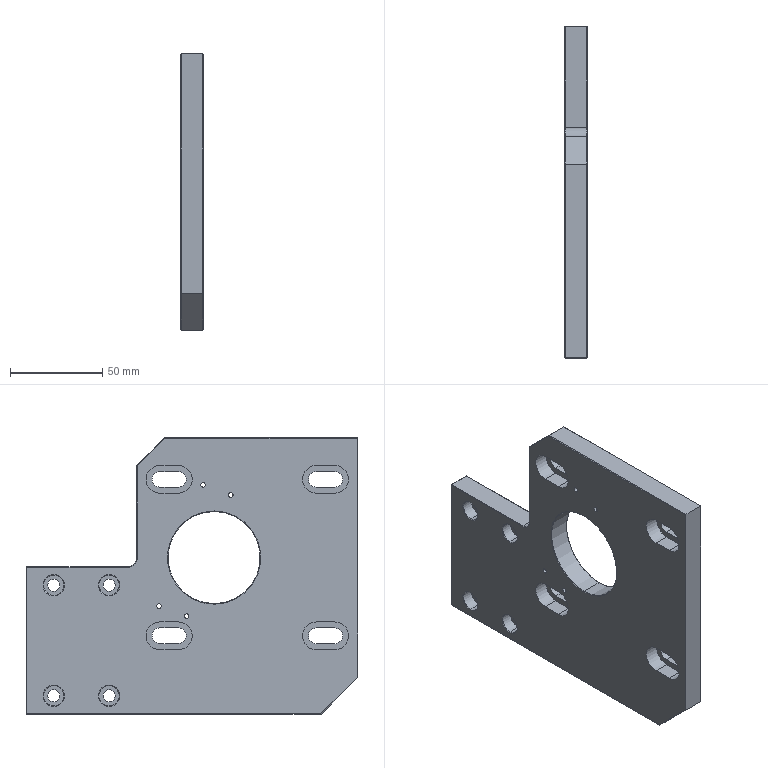Part | STEP file | BPSP-03-011 Motor Fixing Plate2_Default | 1 solid | 121 faces | box 12 x 180 x 150 mm | volume 230112 mm3 | plane 56 | cylinder 43 | cone 22 | commonest cylinder face diameters 2.5 x8 6.6 x8 8.5 x8 11 x8 15 x8 50 x2